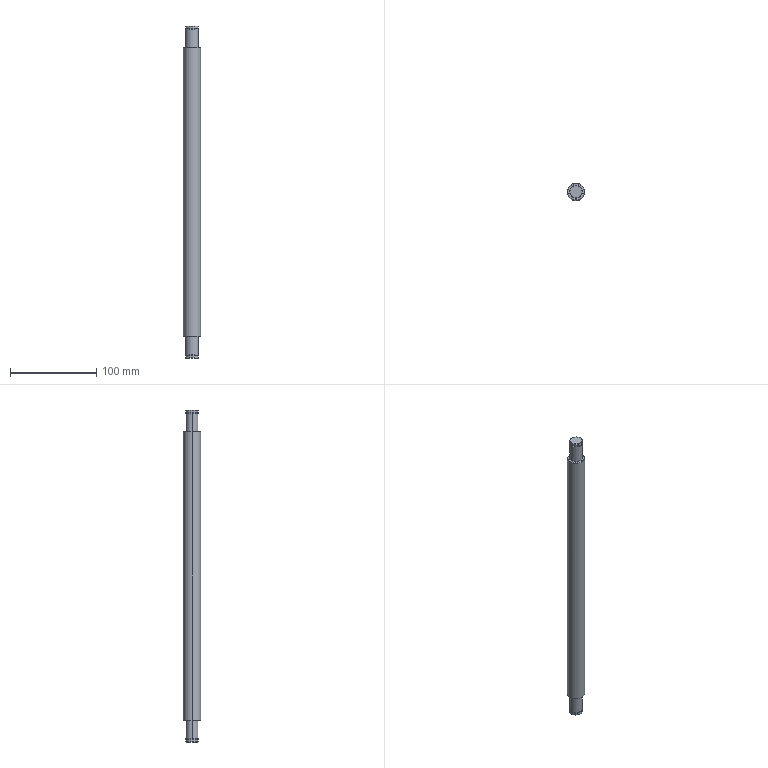Part | STEP file | 倍速链从动轴-0 | 1 solid | 30 faces | box 20 x 20 x 385.3 mm | volume 114081 mm3 | cylinder 14 | cone 8 | plane 8 | commonest cylinder face diameters 15 x8 13.8 x4 20 x2
STEP:
#1=CARTESIAN_POINT('',(-7.,0.,-192.65));
#2=VERTEX_POINT('',#1);
#3=CARTESIAN_POINT('',(7.,0.,-192.65));
#4=VERTEX_POINT('',#3);
#5=CARTESIAN_POINT('',(0.,0.,-192.65));
#6=DIRECTION('',(0.,0.,-1.));
#7=DIRECTION('',(-1.,0.,0.));
#8=AXIS2_PLACEMENT_3D('',#5,#6,#7);
#9=CIRCLE('',#8,7.);
#10=EDGE_CURVE('',#2,#4,#9,.T.);
#11=ORIENTED_EDGE('',*,*,#10,.F.);
#12=CARTESIAN_POINT('',(-7.5,0.,-192.15));
#13=VERTEX_POINT('',#12);
#14=CARTESIAN_POINT('',(-7.,0.,-192.65));
#15=DIRECTION('',(-0.7071,0.,0.7071));
#16=VECTOR('',#15,1000.);
#17=LINE('',#14,#16);
#18=EDGE_CURVE('',#2,#13,#17,.T.);
#19=ORIENTED_EDGE('',*,*,#18,.T.);
#20=CARTESIAN_POINT('',(7.5,0.,-192.15));
#21=VERTEX_POINT('',#20);
#22=CARTESIAN_POINT('',(0.,0.,-192.15));
#23=DIRECTION('',(0.,0.,1.));
#24=DIRECTION('',(-1.,0.,0.));
#25=AXIS2_PLACEMENT_3D('',#22,#23,#24);
#26=CIRCLE('',#25,7.5);
#27=EDGE_CURVE('',#21,#13,#26,.T.);
#28=ORIENTED_EDGE('',*,*,#27,.F.);
#29=CARTESIAN_POINT('',(7.,0.,-192.65));
#30=DIRECTION('',(0.7071,0.,0.7071));
#31=VECTOR('',#30,1000.);
#32=LINE('',#29,#31);
#33=EDGE_CURVE('',#4,#21,#32,.T.);
#34=ORIENTED_EDGE('',*,*,#33,.F.);
#35=EDGE_LOOP('',(#11,#19,#28,#34));
#36=FACE_OUTER_BOUND('',#35,.T.);
#37=CARTESIAN_POINT('',(0.,0.,-192.65));
#38=DIRECTION('',(0.,0.,1.));
#39=DIRECTION('',(1.,0.,0.));
#40=AXIS2_PLACEMENT_3D('',#37,#38,#39);
#41=CONICAL_SURFACE('',#40,7.,0.7854);
#42=ADVANCED_FACE('',(#36),#41,.T.);
#43=CARTESIAN_POINT('',(-9.5,0.,-167.65));
#44=VERTEX_POINT('',#43);
#45=CARTESIAN_POINT('',(9.5,0.,-167.65));
#46=VERTEX_POINT('',#45);
#47=CARTESIAN_POINT('',(0.,0.,-167.65));
#48=DIRECTION('',(0.,0.,-1.));
#49=DIRECTION('',(1.,0.,0.));
#50=AXIS2_PLACEMENT_3D('',#47,#48,#49);
#51=CIRCLE('',#50,9.5);
#52=EDGE_CURVE('',#44,#46,#51,.T.);
#53=ORIENTED_EDGE('',*,*,#52,.F.);
#54=CARTESIAN_POINT('',(-10.,0.,-167.15));
#55=VERTEX_POINT('',#54);
#56=CARTESIAN_POINT('',(-10.,0.,-167.15));
#57=DIRECTION('',(-0.7071,0.,0.7071));
#58=VECTOR('',#57,1000.);
#59=LINE('',#56,#58);
#60=EDGE_CURVE('',#44,#55,#59,.T.);
#61=ORIENTED_EDGE('',*,*,#60,.T.);
#62=CARTESIAN_POINT('',(10.,0.,-167.15));
#63=VERTEX_POINT('',#62);
#64=CARTESIAN_POINT('',(0.,0.,-167.15));
#65=DIRECTION('',(0.,0.,1.));
#66=DIRECTION('',(1.,0.,0.));
#67=AXIS2_PLACEMENT_3D('',#64,#65,#66);
#68=CIRCLE('',#67,10.);
#69=EDGE_CURVE('',#63,#55,#68,.T.);
#70=ORIENTED_EDGE('',*,*,#69,.F.);
#71=CARTESIAN_POINT('',(10.,0.,-167.15));
#72=DIRECTION('',(0.7071,0.,0.7071));
#73=VECTOR('',#72,1000.);
#74=LINE('',#71,#73);
#75=EDGE_CURVE('',#46,#63,#74,.T.);
#76=ORIENTED_EDGE('',*,*,#75,.F.);
#77=EDGE_LOOP('',(#53,#61,#70,#76));
#78=FACE_OUTER_BOUND('',#77,.T.);
#79=CARTESIAN_POINT('',(0.,0.,-167.15));
#80=DIRECTION('',(0.,0.,1.));
#81=DIRECTION('',(1.,0.,0.));
#82=AXIS2_PLACEMENT_3D('',#79,#80,#81);
#83=CONICAL_SURFACE('',#82,10.,0.7854);
#84=ADVANCED_FACE('',(#78),#83,.T.);
#85=CARTESIAN_POINT('',(9.5,0.,167.65));
#86=VERTEX_POINT('',#85);
#87=CARTESIAN_POINT('',(-9.5,0.,167.65));
#88=VERTEX_POINT('',#87);
#89=CARTESIAN_POINT('',(0.,0.,167.65));
#90=DIRECTION('',(0.,0.,1.));
#91=DIRECTION('',(1.,0.,0.));
#92=AXIS2_PLACEMENT_3D('',#89,#90,#91);
#93=CIRCLE('',#92,9.5);
#94=EDGE_CURVE('',#86,#88,#93,.T.);
#95=ORIENTED_EDGE('',*,*,#94,.F.);
#96=CARTESIAN_POINT('',(10.,0.,167.15));
#97=VERTEX_POINT('',#96);
#98=CARTESIAN_POINT('',(9.5,0.,167.65));
#99=DIRECTION('',(0.7071,0.,-0.7071));
#100=VECTOR('',#99,1000.);
#101=LINE('',#98,#100);
#102=EDGE_CURVE('',#86,#97,#101,.T.);
#103=ORIENTED_EDGE('',*,*,#102,.T.);
#104=CARTESIAN_POINT('',(-10.,0.,167.15));
#105=VERTEX_POINT('',#104);
#106=CARTESIAN_POINT('',(0.,0.,167.15));
#107=DIRECTION('',(0.,0.,-1.));
#108=DIRECTION('',(1.,0.,0.));
#109=AXIS2_PLACEMENT_3D('',#106,#107,#108);
#110=CIRCLE('',#109,10.);
#111=EDGE_CURVE('',#105,#97,#110,.T.);
#112=ORIENTED_EDGE('',*,*,#111,.F.);
#113=CARTESIAN_POINT('',(-9.5,0.,167.65));
#114=DIRECTION('',(-0.7071,0.,-0.7071));
#115=VECTOR('',#114,1000.);
#116=LINE('',#113,#115);
#117=EDGE_CURVE('',#88,#105,#116,.T.);
#118=ORIENTED_EDGE('',*,*,#117,.F.);
#119=EDGE_LOOP('',(#95,#103,#112,#118));
#120=FACE_OUTER_BOUND('',#119,.T.);
#121=CARTESIAN_POINT('',(0.,0.,167.65));
#122=DIRECTION('',(0.,0.,-1.));
#123=DIRECTION('',(-1.,0.,0.));
#124=AXIS2_PLACEMENT_3D('',#121,#122,#123);
#125=CONICAL_SURFACE('',#124,9.5,0.7854);
#126=ADVANCED_FACE('',(#120),#125,.T.);
#127=CARTESIAN_POINT('',(7.,0.,192.65));
#128=VERTEX_POINT('',#127);
#129=CARTESIAN_POINT('',(-7.,0.,192.65));
#130=VERTEX_POINT('',#129);
#131=CARTESIAN_POINT('',(0.,0.,192.65));
#132=DIRECTION('',(0.,0.,1.));
#133=DIRECTION('',(1.,0.,0.));
#134=AXIS2_PLACEMENT_3D('',#131,#132,#133);
#135=CIRCLE('',#134,7.);
#136=EDGE_CURVE('',#128,#130,#135,.T.);
#137=ORIENTED_EDGE('',*,*,#136,.F.);
#138=CARTESIAN_POINT('',(7.5,0.,192.15));
#139=VERTEX_POINT('',#138);
#140=CARTESIAN_POINT('',(7.5,0.,192.15));
#141=DIRECTION('',(0.7071,0.,-0.7071));
#142=VECTOR('',#141,1000.);
#143=LINE('',#140,#142);
#144=EDGE_CURVE('',#128,#139,#143,.T.);
#145=ORIENTED_EDGE('',*,*,#144,.T.);
#146=CARTESIAN_POINT('',(-7.5,0.,192.15));
#147=VERTEX_POINT('',#146);
#148=CARTESIAN_POINT('',(0.,0.,192.15));
#149=DIRECTION('',(0.,0.,-1.));
#150=DIRECTION('',(1.,0.,0.));
#151=AXIS2_PLACEMENT_3D('',#148,#149,#150);
#152=CIRCLE('',#151,7.5);
#153=EDGE_CURVE('',#147,#139,#152,.T.);
#154=ORIENTED_EDGE('',*,*,#153,.F.);
#155=CARTESIAN_POINT('',(-7.5,0.,192.15));
#156=DIRECTION('',(-0.7071,0.,-0.7071));
#157=VECTOR('',#156,1000.);
#158=LINE('',#155,#157);
#159=EDGE_CURVE('',#130,#147,#158,.T.);
#160=ORIENTED_EDGE('',*,*,#159,.F.);
#161=EDGE_LOOP('',(#137,#145,#154,#160));
#162=FACE_OUTER_BOUND('',#161,.T.);
#163=CARTESIAN_POINT('',(0.,0.,192.15));
#164=DIRECTION('',(0.,0.,-1.));
#165=DIRECTION('',(-1.,0.,0.));
#166=AXIS2_PLACEMENT_3D('',#163,#164,#165);
#167=CONICAL_SURFACE('',#166,7.5,0.7854);
#168=ADVANCED_FACE('',(#162),#167,.T.);
#169=ORIENTED_EDGE('',*,*,#27,.T.);
#170=CARTESIAN_POINT('',(-7.5,0.,-189.85));
#171=VERTEX_POINT('',#170);
#172=CARTESIAN_POINT('',(-7.5,0.,-192.65));
#173=DIRECTION('',(0.,0.,1.));
#174=VECTOR('',#173,1000.);
#175=LINE('',#172,#174);
#176=EDGE_CURVE('',#13,#171,#175,.T.);
#177=ORIENTED_EDGE('',*,*,#176,.T.);
#178=CARTESIAN_POINT('',(7.5,0.,-189.85));
#179=VERTEX_POINT('',#178);
#180=CARTESIAN_POINT('',(0.,0.,-189.85));
#181=DIRECTION('',(0.,0.,-1.));
#182=DIRECTION('',(-1.,0.,0.));
#183=AXIS2_PLACEMENT_3D('',#180,#181,#182);
#184=CIRCLE('',#183,7.5);
#185=EDGE_CURVE('',#171,#179,#184,.T.);
#186=ORIENTED_EDGE('',*,*,#185,.T.);
#187=CARTESIAN_POINT('',(7.5,0.,-192.65));
#188=DIRECTION('',(0.,0.,1.));
#189=VECTOR('',#188,1000.);
#190=LINE('',#187,#189);
#191=EDGE_CURVE('',#21,#179,#190,.T.);
#192=ORIENTED_EDGE('',*,*,#191,.F.);
#193=EDGE_LOOP('',(#169,#177,#186,#192));
#194=FACE_OUTER_BOUND('',#193,.T.);
#195=CARTESIAN_POINT('',(0.,0.,-192.65));
#196=DIRECTION('',(0.,0.,1.));
#197=DIRECTION('',(1.,0.,0.));
#198=AXIS2_PLACEMENT_3D('',#195,#196,#197);
#199=CYLINDRICAL_SURFACE('',#198,7.5);
#200=ADVANCED_FACE('',(#194),#199,.T.);
#201=CARTESIAN_POINT('',(6.9,0.,-189.85));
#202=VERTEX_POINT('',#201);
#203=CARTESIAN_POINT('',(-6.9,0.,-189.85));
#204=VERTEX_POINT('',#203);
#205=CARTESIAN_POINT('',(0.,0.,-189.85));
#206=DIRECTION('',(0.,0.,-1.));
#207=DIRECTION('',(-1.,0.,0.));
#208=AXIS2_PLACEMENT_3D('',#205,#206,#207);
#209=CIRCLE('',#208,6.9);
#210=EDGE_CURVE('',#202,#204,#209,.T.);
#211=ORIENTED_EDGE('',*,*,#210,.F.);
#212=CARTESIAN_POINT('',(6.9,0.,-188.65));
#213=VERTEX_POINT('',#212);
#214=CARTESIAN_POINT('',(6.9,0.,0.));
#215=DIRECTION('',(0.,0.,1.));
#216=VECTOR('',#215,1000.);
#217=LINE('',#214,#216);
#218=EDGE_CURVE('',#202,#213,#217,.T.);
#219=ORIENTED_EDGE('',*,*,#218,.T.);
#220=CARTESIAN_POINT('',(-6.9,0.,-188.65));
#221=VERTEX_POINT('',#220);
#222=CARTESIAN_POINT('',(0.,0.,-188.65));
#223=DIRECTION('',(0.,0.,-1.));
#224=DIRECTION('',(-1.,0.,0.));
#225=AXIS2_PLACEMENT_3D('',#222,#223,#224);
#226=CIRCLE('',#225,6.9);
#227=EDGE_CURVE('',#213,#221,#226,.T.);
#228=ORIENTED_EDGE('',*,*,#227,.T.);
#229=CARTESIAN_POINT('',(-6.9,0.,0.));
#230=DIRECTION('',(0.,0.,1.));
#231=VECTOR('',#230,1000.);
#232=LINE('',#229,#231);
#233=EDGE_CURVE('',#204,#221,#232,.T.);
#234=ORIENTED_EDGE('',*,*,#233,.F.);
#235=EDGE_LOOP('',(#211,#219,#228,#234));
#236=FACE_OUTER_BOUND('',#235,.T.);
#237=CARTESIAN_POINT('',(0.,0.,0.));
#238=DIRECTION('',(0.,0.,1.));
#239=DIRECTION('',(-1.,0.,0.));
#240=AXIS2_PLACEMENT_3D('',#237,#238,#239);
#241=CYLINDRICAL_SURFACE('',#240,6.9);
#242=ADVANCED_FACE('',(#236),#241,.T.);
#243=ORIENTED_EDGE('',*,*,#153,.T.);
#244=CARTESIAN_POINT('',(7.5,0.,189.85));
#245=VERTEX_POINT('',#244);
#246=CARTESIAN_POINT('',(7.5,0.,192.65));
#247=DIRECTION('',(0.,0.,-1.));
#248=VECTOR('',#247,1000.);
#249=LINE('',#246,#248);
#250=EDGE_CURVE('',#139,#245,#249,.T.);
#251=ORIENTED_EDGE('',*,*,#250,.T.);
#252=CARTESIAN_POINT('',(-7.5,0.,189.85));
#253=VERTEX_POINT('',#252);
#254=CARTESIAN_POINT('',(0.,0.,189.85));
#255=DIRECTION('',(0.,0.,-1.));
#256=DIRECTION('',(1.,0.,0.));
#257=AXIS2_PLACEMENT_3D('',#254,#255,#256);
#258=CIRCLE('',#257,7.5);
#259=EDGE_CURVE('',#253,#245,#258,.T.);
#260=ORIENTED_EDGE('',*,*,#259,.F.);
#261=CARTESIAN_POINT('',(-7.5,0.,192.65));
#262=DIRECTION('',(0.,0.,-1.));
#263=VECTOR('',#262,1000.);
#264=LINE('',#261,#263);
#265=EDGE_CURVE('',#147,#253,#264,.T.);
#266=ORIENTED_EDGE('',*,*,#265,.F.);
#267=EDGE_LOOP('',(#243,#251,#260,#266));
#268=FACE_OUTER_BOUND('',#267,.T.);
#269=CARTESIAN_POINT('',(0.,0.,192.65));
#270=DIRECTION('',(0.,0.,-1.));
#271=DIRECTION('',(-1.,0.,0.));
#272=AXIS2_PLACEMENT_3D('',#269,#270,#271);
#273=CYLINDRICAL_SURFACE('',#272,7.5);
#274=ADVANCED_FACE('',(#268),#273,.T.);
#275=CARTESIAN_POINT('',(-6.9,0.,189.85));
#276=VERTEX_POINT('',#275);
#277=CARTESIAN_POINT('',(6.9,0.,189.85));
#278=VERTEX_POINT('',#277);
#279=CARTESIAN_POINT('',(0.,0.,189.85));
#280=DIRECTION('',(0.,0.,-1.));
#281=DIRECTION('',(-1.,0.,0.));
#282=AXIS2_PLACEMENT_3D('',#279,#280,#281);
#283=CIRCLE('',#282,6.9);
#284=EDGE_CURVE('',#276,#278,#283,.T.);
#285=ORIENTED_EDGE('',*,*,#284,.T.);
#286=CARTESIAN_POINT('',(6.9,0.,188.65));
#287=VERTEX_POINT('',#286);
#288=CARTESIAN_POINT('',(6.9,0.,0.));
#289=DIRECTION('',(0.,0.,-1.));
#290=VECTOR('',#289,1000.);
#291=LINE('',#288,#290);
#292=EDGE_CURVE('',#278,#287,#291,.T.);
#293=ORIENTED_EDGE('',*,*,#292,.T.);
#294=CARTESIAN_POINT('',(-6.9,0.,188.65));
#295=VERTEX_POINT('',#294);
#296=CARTESIAN_POINT('',(0.,0.,188.65));
#297=DIRECTION('',(0.,0.,-1.));
#298=DIRECTION('',(-1.,0.,0.));
#299=AXIS2_PLACEMENT_3D('',#296,#297,#298);
#300=CIRCLE('',#299,6.9);
#301=EDGE_CURVE('',#295,#287,#300,.T.);
#302=ORIENTED_EDGE('',*,*,#301,.F.);
#303=CARTESIAN_POINT('',(-6.9,0.,0.));
#304=DIRECTION('',(0.,0.,-1.));
#305=VECTOR('',#304,1000.);
#306=LINE('',#303,#305);
#307=EDGE_CURVE('',#276,#295,#306,.T.);
#308=ORIENTED_EDGE('',*,*,#307,.F.);
#309=EDGE_LOOP('',(#285,#293,#302,#308));
#310=FACE_OUTER_BOUND('',#309,.T.);
#311=CARTESIAN_POINT('',(0.,0.,0.));
#312=DIRECTION('',(0.,0.,-1.));
#313=DIRECTION('',(-1.,0.,0.));
#314=AXIS2_PLACEMENT_3D('',#311,#312,#313);
#315=CYLINDRICAL_SURFACE('',#314,6.9);
#316=ADVANCED_FACE('',(#310),#315,.T.);
#317=CARTESIAN_POINT('',(7.5,0.,188.65));
#318=VERTEX_POINT('',#317);
#319=CARTESIAN_POINT('',(-7.5,0.,188.65));
#320=VERTEX_POINT('',#319);
#321=CARTESIAN_POINT('',(0.,0.,188.65));
#322=DIRECTION('',(0.,0.,1.));
#323=DIRECTION('',(-1.,0.,0.));
#324=AXIS2_PLACEMENT_3D('',#321,#322,#323);
#325=CIRCLE('',#324,7.5);
#326=EDGE_CURVE('',#318,#320,#325,.T.);
#327=ORIENTED_EDGE('',*,*,#326,.F.);
#328=CARTESIAN_POINT('',(7.5,0.,167.65));
#329=VERTEX_POINT('',#328);
#330=CARTESIAN_POINT('',(7.5,0.,192.65));
#331=DIRECTION('',(0.,0.,-1.));
#332=VECTOR('',#331,1000.);
#333=LINE('',#330,#332);
#334=EDGE_CURVE('',#318,#329,#333,.T.);
#335=ORIENTED_EDGE('',*,*,#334,.T.);
#336=CARTESIAN_POINT('',(-7.5,0.,167.65));
#337=VERTEX_POINT('',#336);
#338=CARTESIAN_POINT('',(0.,0.,167.65));
#339=DIRECTION('',(0.,0.,1.));
#340=DIRECTION('',(1.,0.,0.));
#341=AXIS2_PLACEMENT_3D('',#338,#339,#340);
#342=CIRCLE('',#341,7.5);
#343=EDGE_CURVE('',#329,#337,#342,.T.);
#344=ORIENTED_EDGE('',*,*,#343,.T.);
#345=CARTESIAN_POINT('',(-7.5,0.,192.65));
#346=DIRECTION('',(0.,0.,-1.));
#347=VECTOR('',#346,1000.);
#348=LINE('',#345,#347);
#349=EDGE_CURVE('',#320,#337,#348,.T.);
#350=ORIENTED_EDGE('',*,*,#349,.F.);
#351=EDGE_LOOP('',(#327,#335,#344,#350));
#352=FACE_OUTER_BOUND('',#351,.T.);
#353=CARTESIAN_POINT('',(0.,0.,192.65));
#354=DIRECTION('',(0.,0.,-1.));
#355=DIRECTION('',(-1.,0.,0.));
#356=AXIS2_PLACEMENT_3D('',#353,#354,#355);
#357=CYLINDRICAL_SURFACE('',#356,7.5);
#358=ADVANCED_FACE('',(#352),#357,.T.);
#359=CARTESIAN_POINT('',(7.5,0.,-188.65));
#360=VERTEX_POINT('',#359);
#361=CARTESIAN_POINT('',(-7.5,0.,-188.65));
#362=VERTEX_POINT('',#361);
#363=CARTESIAN_POINT('',(0.,0.,-188.65));
#364=DIRECTION('',(0.,0.,1.));
#365=DIRECTION('',(1.,0.,0.));
#366=AXIS2_PLACEMENT_3D('',#363,#364,#365);
#367=CIRCLE('',#366,7.5);
#368=EDGE_CURVE('',#360,#362,#367,.T.);
#369=ORIENTED_EDGE('',*,*,#368,.T.);
#370=CARTESIAN_POINT('',(-7.5,0.,-167.65));
#371=VERTEX_POINT('',#370);
#372=CARTESIAN_POINT('',(-7.5,0.,-192.65));
#373=DIRECTION('',(0.,0.,1.));
#374=VECTOR('',#373,1000.);
#375=LINE('',#372,#374);
#376=EDGE_CURVE('',#362,#371,#375,.T.);
#377=ORIENTED_EDGE('',*,*,#376,.T.);
#378=CARTESIAN_POINT('',(7.5,0.,-167.65));
#379=VERTEX_POINT('',#378);
#380=CARTESIAN_POINT('',(0.,0.,-167.65));
#381=DIRECTION('',(0.,0.,-1.));
#382=DIRECTION('',(1.,0.,0.));
#383=AXIS2_PLACEMENT_3D('',#380,#381,#382);
#384=CIRCLE('',#383,7.5);
#385=EDGE_CURVE('',#371,#379,#384,.T.);
#386=ORIENTED_EDGE('',*,*,#385,.T.);
#387=CARTESIAN_POINT('',(7.5,0.,-192.65));
#388=DIRECTION('',(0.,0.,1.));
#389=VECTOR('',#388,1000.);
#390=LINE('',#387,#389);
#391=EDGE_CURVE('',#360,#379,#390,.T.);
#392=ORIENTED_EDGE('',*,*,#391,.F.);
#393=EDGE_LOOP('',(#369,#377,#386,#392));
#394=FACE_OUTER_BOUND('',#393,.T.);
#395=CARTESIAN_POINT('',(0.,0.,-192.65));
#396=DIRECTION('',(0.,0.,1.));
#397=DIRECTION('',(1.,0.,0.));
#398=AXIS2_PLACEMENT_3D('',#395,#396,#397);
#399=CYLINDRICAL_SURFACE('',#398,7.5);
#400=ADVANCED_FACE('',(#394),#399,.T.);
#401=ORIENTED_EDGE('',*,*,#111,.T.);
#402=CARTESIAN_POINT('',(10.,0.,167.65));
#403=DIRECTION('',(0.,0.,-1.));
#404=VECTOR('',#403,1000.);
#405=LINE('',#402,#404);
#406=EDGE_CURVE('',#97,#63,#405,.T.);
#407=ORIENTED_EDGE('',*,*,#406,.T.);
#408=ORIENTED_EDGE('',*,*,#69,.T.);
#409=CARTESIAN_POINT('',(-10.,0.,167.65));
#410=DIRECTION('',(0.,0.,-1.));
#411=VECTOR('',#410,1000.);
#412=LINE('',#409,#411);
#413=EDGE_CURVE('',#105,#55,#412,.T.);
#414=ORIENTED_EDGE('',*,*,#413,.F.);
#415=EDGE_LOOP('',(#401,#407,#408,#414));
#416=FACE_OUTER_BOUND('',#415,.T.);
#417=CARTESIAN_POINT('',(0.,0.,167.65));
#418=DIRECTION('',(0.,0.,-1.));
#419=DIRECTION('',(-1.,0.,0.));
#420=AXIS2_PLACEMENT_3D('',#417,#418,#419);
#421=CYLINDRICAL_SURFACE('',#420,10.);
#422=ADVANCED_FACE('',(#416),#421,.T.);
#423=CARTESIAN_POINT('',(0.,0.,-167.65));
#424=DIRECTION('',(0.,0.,-1.));
#425=DIRECTION('',(1.,0.,0.));
#426=AXIS2_PLACEMENT_3D('',#423,#424,#425);
#427=CIRCLE('',#426,9.5);
#428=EDGE_CURVE('',#46,#44,#427,.T.);
#429=ORIENTED_EDGE('',*,*,#428,.T.);
#430=ORIENTED_EDGE('',*,*,#52,.T.);
#431=EDGE_LOOP('',(#429,#430));
#432=FACE_OUTER_BOUND('',#431,.T.);
#433=CARTESIAN_POINT('',(0.,0.,-167.65));
#434=DIRECTION('',(0.,0.,-1.));
#435=DIRECTION('',(1.,0.,0.));
#436=AXIS2_PLACEMENT_3D('',#433,#434,#435);
#437=CIRCLE('',#436,7.5);
#438=EDGE_CURVE('',#379,#371,#437,.T.);
#439=ORIENTED_EDGE('',*,*,#438,.F.);
#440=ORIENTED_EDGE('',*,*,#385,.F.);
#441=EDGE_LOOP('',(#439,#440));
#442=FACE_BOUND('',#441,.T.);
#443=CARTESIAN_POINT('',(0.,0.,-167.65));
#444=DIRECTION('',(0.,0.,1.));
#445=DIRECTION('',(1.,0.,0.));
#446=AXIS2_PLACEMENT_3D('',#443,#444,#445);
#447=PLANE('',#446);
#448=ADVANCED_FACE('',(#432,#442),#447,.F.);
#449=ORIENTED_EDGE('',*,*,#406,.F.);
#450=CARTESIAN_POINT('',(0.,0.,167.15));
#451=DIRECTION('',(0.,0.,-1.));
#452=DIRECTION('',(1.,0.,0.));
#453=AXIS2_PLACEMENT_3D('',#450,#451,#452);
#454=CIRCLE('',#453,10.);
#455=EDGE_CURVE('',#97,#105,#454,.T.);
#456=ORIENTED_EDGE('',*,*,#455,.T.);
#457=ORIENTED_EDGE('',*,*,#413,.T.);
#458=CARTESIAN_POINT('',(0.,0.,-167.15));
#459=DIRECTION('',(0.,0.,1.));
#460=DIRECTION('',(1.,0.,0.));
#461=AXIS2_PLACEMENT_3D('',#458,#459,#460);
#462=CIRCLE('',#461,10.);
#463=EDGE_CURVE('',#55,#63,#462,.T.);
#464=ORIENTED_EDGE('',*,*,#463,.T.);
#465=EDGE_LOOP('',(#449,#456,#457,#464));
#466=FACE_OUTER_BOUND('',#465,.T.);
#467=CARTESIAN_POINT('',(0.,0.,167.65));
#468=DIRECTION('',(0.,0.,-1.));
#469=DIRECTION('',(-1.,0.,0.));
#470=AXIS2_PLACEMENT_3D('',#467,#468,#469);
#471=CYLINDRICAL_SURFACE('',#470,10.);
#472=ADVANCED_FACE('',(#466),#471,.T.);
#473=CARTESIAN_POINT('',(0.,0.,167.65));
#474=DIRECTION('',(0.,0.,1.));
#475=DIRECTION('',(1.,0.,0.));
#476=AXIS2_PLACEMENT_3D('',#473,#474,#475);
#477=CIRCLE('',#476,9.5);
#478=EDGE_CURVE('',#88,#86,#477,.T.);
#479=ORIENTED_EDGE('',*,*,#478,.T.);
#480=ORIENTED_EDGE('',*,*,#94,.T.);
#481=EDGE_LOOP('',(#479,#480));
#482=FACE_OUTER_BOUND('',#481,.T.);
#483=CARTESIAN_POINT('',(0.,0.,167.65));
#484=DIRECTION('',(0.,0.,1.));
#485=DIRECTION('',(1.,0.,0.));
#486=AXIS2_PLACEMENT_3D('',#483,#484,#485);
#487=CIRCLE('',#486,7.5);
#488=EDGE_CURVE('',#337,#329,#487,.T.);
#489=ORIENTED_EDGE('',*,*,#488,.F.);
#490=ORIENTED_EDGE('',*,*,#343,.F.);
#491=EDGE_LOOP('',(#489,#490));
#492=FACE_BOUND('',#491,.T.);
#493=CARTESIAN_POINT('',(0.,0.,167.65));
#494=DIRECTION('',(0.,0.,1.));
#495=DIRECTION('',(1.,0.,0.));
#496=AXIS2_PLACEMENT_3D('',#493,#494,#495);
#497=PLANE('',#496);
#498=ADVANCED_FACE('',(#482,#492),#497,.T.);
#499=ORIENTED_EDGE('',*,*,#376,.F.);
#500=CARTESIAN_POINT('',(0.,0.,-188.65));
#501=DIRECTION('',(0.,0.,1.));
#502=DIRECTION('',(1.,0.,0.));
#503=AXIS2_PLACEMENT_3D('',#500,#501,#502);
#504=CIRCLE('',#503,7.5);
#505=EDGE_CURVE('',#362,#360,#504,.T.);
#506=ORIENTED_EDGE('',*,*,#505,.T.);
#507=ORIENTED_EDGE('',*,*,#391,.T.);
#508=ORIENTED_EDGE('',*,*,#438,.T.);
#509=EDGE_LOOP('',(#499,#506,#507,#508));
#510=FACE_OUTER_BOUND('',#509,.T.);
#511=CARTESIAN_POINT('',(0.,0.,-192.65));
#512=DIRECTION('',(0.,0.,1.));
#513=DIRECTION('',(1.,0.,0.));
#514=AXIS2_PLACEMENT_3D('',#511,#512,#513);
#515=CYLINDRICAL_SURFACE('',#514,7.5);
#516=ADVANCED_FACE('',(#510),#515,.T.);
#517=ORIENTED_EDGE('',*,*,#334,.F.);
#518=CARTESIAN_POINT('',(0.,0.,188.65));
#519=DIRECTION('',(0.,0.,1.));
#520=DIRECTION('',(-1.,0.,0.));
#521=AXIS2_PLACEMENT_3D('',#518,#519,#520);
#522=CIRCLE('',#521,7.5);
#523=EDGE_CURVE('',#320,#318,#522,.T.);
#524=ORIENTED_EDGE('',*,*,#523,.F.);
#525=ORIENTED_EDGE('',*,*,#349,.T.);
#526=ORIENTED_EDGE('',*,*,#488,.T.);
#527=EDGE_LOOP('',(#517,#524,#525,#526));
#528=FACE_OUTER_BOUND('',#527,.T.);
#529=CARTESIAN_POINT('',(0.,0.,192.65));
#530=DIRECTION('',(0.,0.,-1.));
#531=DIRECTION('',(-1.,0.,0.));
#532=AXIS2_PLACEMENT_3D('',#529,#530,#531);
#533=CYLINDRICAL_SURFACE('',#532,7.5);
#534=ADVANCED_FACE('',(#528),#533,.T.);
#535=ORIENTED_EDGE('',*,*,#259,.T.);
#536=CARTESIAN_POINT('',(0.,0.,189.85));
#537=DIRECTION('',(0.,0.,-1.));
#538=DIRECTION('',(1.,0.,0.));
#539=AXIS2_PLACEMENT_3D('',#536,#537,#538);
#540=CIRCLE('',#539,7.5);
#541=EDGE_CURVE('',#245,#253,#540,.T.);
#542=ORIENTED_EDGE('',*,*,#541,.T.);
#543=EDGE_LOOP('',(#535,#542));
#544=FACE_OUTER_BOUND('',#543,.T.);
#545=ORIENTED_EDGE('',*,*,#284,.F.);
#546=CARTESIAN_POINT('',(0.,0.,189.85));
#547=DIRECTION('',(0.,0.,-1.));
#548=DIRECTION('',(-1.,0.,0.));
#549=AXIS2_PLACEMENT_3D('',#546,#547,#548);
#550=CIRCLE('',#549,6.9);
#551=EDGE_CURVE('',#278,#276,#550,.T.);
#552=ORIENTED_EDGE('',*,*,#551,.F.);
#553=EDGE_LOOP('',(#545,#552));
#554=FACE_BOUND('',#553,.T.);
#555=CARTESIAN_POINT('',(-11.9,0.,189.85));
#556=DIRECTION('',(0.,0.,1.));
#557=DIRECTION('',(1.,0.,0.));
#558=AXIS2_PLACEMENT_3D('',#555,#556,#557);
#559=PLANE('',#558);
#560=ADVANCED_FACE('',(#544,#554),#559,.F.);
#561=ORIENTED_EDGE('',*,*,#292,.F.);
#562=ORIENTED_EDGE('',*,*,#551,.T.);
#563=ORIENTED_EDGE('',*,*,#307,.T.);
#564=CARTESIAN_POINT('',(0.,0.,188.65));
#565=DIRECTION('',(0.,0.,-1.));
#566=DIRECTION('',(-1.,0.,0.));
#567=AXIS2_PLACEMENT_3D('',#564,#565,#566);
#568=CIRCLE('',#567,6.9);
#569=EDGE_CURVE('',#287,#295,#568,.T.);
#570=ORIENTED_EDGE('',*,*,#569,.F.);
#571=EDGE_LOOP('',(#561,#562,#563,#570));
#572=FACE_OUTER_BOUND('',#571,.T.);
#573=CARTESIAN_POINT('',(0.,0.,0.));
#574=DIRECTION('',(0.,0.,-1.));
#575=DIRECTION('',(-1.,0.,0.));
#576=AXIS2_PLACEMENT_3D('',#573,#574,#575);
#577=CYLINDRICAL_SURFACE('',#576,6.9);
#578=ADVANCED_FACE('',(#572),#577,.T.);
#579=ORIENTED_EDGE('',*,*,#523,.T.);
#580=ORIENTED_EDGE('',*,*,#326,.T.);
#581=EDGE_LOOP('',(#579,#580));
#582=FACE_OUTER_BOUND('',#581,.T.);
#583=ORIENTED_EDGE('',*,*,#301,.T.);
#584=ORIENTED_EDGE('',*,*,#569,.T.);
#585=EDGE_LOOP('',(#583,#584));
#586=FACE_BOUND('',#585,.T.);
#587=CARTESIAN_POINT('',(-11.9,0.,188.65));
#588=DIRECTION('',(0.,0.,-1.));
#589=DIRECTION('',(-1.,0.,0.));
#590=AXIS2_PLACEMENT_3D('',#587,#588,#589);
#591=PLANE('',#590);
#592=ADVANCED_FACE('',(#582,#586),#591,.F.);
#593=CARTESIAN_POINT('',(0.,0.,192.65));
#594=DIRECTION('',(0.,0.,1.));
#595=DIRECTION('',(1.,0.,0.));
#596=AXIS2_PLACEMENT_3D('',#593,#594,#595);
#597=CIRCLE('',#596,7.);
#598=EDGE_CURVE('',#130,#128,#597,.T.);
#599=ORIENTED_EDGE('',*,*,#598,.T.);
#600=ORIENTED_EDGE('',*,*,#136,.T.);
#601=EDGE_LOOP('',(#599,#600));
#602=FACE_OUTER_BOUND('',#601,.T.);
#603=CARTESIAN_POINT('',(0.,0.,192.65));
#604=DIRECTION('',(0.,0.,1.));
#605=DIRECTION('',(-1.,0.,0.));
#606=AXIS2_PLACEMENT_3D('',#603,#604,#605);
#607=PLANE('',#606);
#608=ADVANCED_FACE('',(#602),#607,.T.);
#609=ORIENTED_EDGE('',*,*,#250,.F.);
#610=CARTESIAN_POINT('',(0.,0.,192.15));
#611=DIRECTION('',(0.,0.,-1.));
#612=DIRECTION('',(1.,0.,0.));
#613=AXIS2_PLACEMENT_3D('',#610,#611,#612);
#614=CIRCLE('',#613,7.5);
#615=EDGE_CURVE('',#139,#147,#614,.T.);
#616=ORIENTED_EDGE('',*,*,#615,.T.);
#617=ORIENTED_EDGE('',*,*,#265,.T.);
#618=ORIENTED_EDGE('',*,*,#541,.F.);
#619=EDGE_LOOP('',(#609,#616,#617,#618));
#620=FACE_OUTER_BOUND('',#619,.T.);
#621=CARTESIAN_POINT('',(0.,0.,192.65));
#622=DIRECTION('',(0.,0.,-1.));
#623=DIRECTION('',(-1.,0.,0.));
#624=AXIS2_PLACEMENT_3D('',#621,#622,#623);
#625=CYLINDRICAL_SURFACE('',#624,7.5);
#626=ADVANCED_FACE('',(#620),#625,.T.);
#627=CARTESIAN_POINT('',(0.,0.,-189.85));
#628=DIRECTION('',(0.,0.,-1.));
#629=DIRECTION('',(-1.,0.,0.));
#630=AXIS2_PLACEMENT_3D('',#627,#628,#629);
#631=CIRCLE('',#630,6.9);
#632=EDGE_CURVE('',#204,#202,#631,.T.);
#633=ORIENTED_EDGE('',*,*,#632,.T.);
#634=ORIENTED_EDGE('',*,*,#210,.T.);
#635=EDGE_LOOP('',(#633,#634));
#636=FACE_BOUND('',#635,.T.);
#637=CARTESIAN_POINT('',(0.,0.,-189.85));
#638=DIRECTION('',(0.,0.,-1.));
#639=DIRECTION('',(-1.,0.,0.));
#640=AXIS2_PLACEMENT_3D('',#637,#638,#639);
#641=CIRCLE('',#640,7.5);
#642=EDGE_CURVE('',#179,#171,#641,.T.);
#643=ORIENTED_EDGE('',*,*,#642,.F.);
#644=ORIENTED_EDGE('',*,*,#185,.F.);
#645=EDGE_LOOP('',(#643,#644));
#646=FACE_OUTER_BOUND('',#645,.T.);
#647=CARTESIAN_POINT('',(-11.9,0.,-189.85));
#648=DIRECTION('',(0.,0.,-1.));
#649=DIRECTION('',(1.,0.,0.));
#650=AXIS2_PLACEMENT_3D('',#647,#648,#649);
#651=PLANE('',#650);
#652=ADVANCED_FACE('',(#636,#646),#651,.F.);
#653=CARTESIAN_POINT('',(0.,0.,-188.65));
#654=DIRECTION('',(0.,0.,-1.));
#655=DIRECTION('',(-1.,0.,0.));
#656=AXIS2_PLACEMENT_3D('',#653,#654,#655);
#657=CIRCLE('',#656,6.9);
#658=EDGE_CURVE('',#221,#213,#657,.T.);
#659=ORIENTED_EDGE('',*,*,#658,.F.);
#660=ORIENTED_EDGE('',*,*,#227,.F.);
#661=EDGE_LOOP('',(#659,#660));
#662=FACE_BOUND('',#661,.T.);
#663=ORIENTED_EDGE('',*,*,#368,.F.);
#664=ORIENTED_EDGE('',*,*,#505,.F.);
#665=EDGE_LOOP('',(#663,#664));
#666=FACE_OUTER_BOUND('',#665,.T.);
#667=CARTESIAN_POINT('',(-11.9,0.,-188.65));
#668=DIRECTION('',(0.,0.,1.));
#669=DIRECTION('',(-1.,0.,0.));
#670=AXIS2_PLACEMENT_3D('',#667,#668,#669);
#671=PLANE('',#670);
#672=ADVANCED_FACE('',(#662,#666),#671,.F.);
#673=ORIENTED_EDGE('',*,*,#218,.F.);
#674=ORIENTED_EDGE('',*,*,#632,.F.);
#675=ORIENTED_EDGE('',*,*,#233,.T.);
#676=ORIENTED_EDGE('',*,*,#658,.T.);
#677=EDGE_LOOP('',(#673,#674,#675,#676));
#678=FACE_OUTER_BOUND('',#677,.T.);
#679=CARTESIAN_POINT('',(0.,0.,0.));
#680=DIRECTION('',(0.,0.,1.));
#681=DIRECTION('',(-1.,0.,0.));
#682=AXIS2_PLACEMENT_3D('',#679,#680,#681);
#683=CYLINDRICAL_SURFACE('',#682,6.9);
#684=ADVANCED_FACE('',(#678),#683,.T.);
#685=CARTESIAN_POINT('',(0.,0.,-192.65));
#686=DIRECTION('',(0.,0.,-1.));
#687=DIRECTION('',(-1.,0.,0.));
#688=AXIS2_PLACEMENT_3D('',#685,#686,#687);
#689=CIRCLE('',#688,7.);
#690=EDGE_CURVE('',#4,#2,#689,.T.);
#691=ORIENTED_EDGE('',*,*,#690,.T.);
#692=ORIENTED_EDGE('',*,*,#10,.T.);
#693=EDGE_LOOP('',(#691,#692));
#694=FACE_OUTER_BOUND('',#693,.T.);
#695=CARTESIAN_POINT('',(0.,0.,-192.65));
#696=DIRECTION('',(0.,0.,-1.));
#697=DIRECTION('',(-1.,0.,0.));
#698=AXIS2_PLACEMENT_3D('',#695,#696,#697);
#699=PLANE('',#698);
#700=ADVANCED_FACE('',(#694),#699,.T.);
#701=ORIENTED_EDGE('',*,*,#176,.F.);
#702=CARTESIAN_POINT('',(0.,0.,-192.15));
#703=DIRECTION('',(0.,0.,1.));
#704=DIRECTION('',(-1.,0.,0.));
#705=AXIS2_PLACEMENT_3D('',#702,#703,#704);
#706=CIRCLE('',#705,7.5);
#707=EDGE_CURVE('',#13,#21,#706,.T.);
#708=ORIENTED_EDGE('',*,*,#707,.T.);
#709=ORIENTED_EDGE('',*,*,#191,.T.);
#710=ORIENTED_EDGE('',*,*,#642,.T.);
#711=EDGE_LOOP('',(#701,#708,#709,#710));
#712=FACE_OUTER_BOUND('',#711,.T.);
#713=CARTESIAN_POINT('',(0.,0.,-192.65));
#714=DIRECTION('',(0.,0.,1.));
#715=DIRECTION('',(1.,0.,0.));
#716=AXIS2_PLACEMENT_3D('',#713,#714,#715);
#717=CYLINDRICAL_SURFACE('',#716,7.5);
#718=ADVANCED_FACE('',(#712),#717,.T.);
#719=ORIENTED_EDGE('',*,*,#144,.F.);
#720=ORIENTED_EDGE('',*,*,#598,.F.);
#721=ORIENTED_EDGE('',*,*,#159,.T.);
#722=ORIENTED_EDGE('',*,*,#615,.F.);
#723=EDGE_LOOP('',(#719,#720,#721,#722));
#724=FACE_OUTER_BOUND('',#723,.T.);
#725=CARTESIAN_POINT('',(0.,0.,192.15));
#726=DIRECTION('',(0.,0.,-1.));
#727=DIRECTION('',(-1.,0.,0.));
#728=AXIS2_PLACEMENT_3D('',#725,#726,#727);
#729=CONICAL_SURFACE('',#728,7.5,0.7854);
#730=ADVANCED_FACE('',(#724),#729,.T.);
#731=ORIENTED_EDGE('',*,*,#102,.F.);
#732=ORIENTED_EDGE('',*,*,#478,.F.);
#733=ORIENTED_EDGE('',*,*,#117,.T.);
#734=ORIENTED_EDGE('',*,*,#455,.F.);
#735=EDGE_LOOP('',(#731,#732,#733,#734));
#736=FACE_OUTER_BOUND('',#735,.T.);
#737=CARTESIAN_POINT('',(0.,0.,167.65));
#738=DIRECTION('',(0.,0.,-1.));
#739=DIRECTION('',(-1.,0.,0.));
#740=AXIS2_PLACEMENT_3D('',#737,#738,#739);
#741=CONICAL_SURFACE('',#740,9.5,0.7854);
#742=ADVANCED_FACE('',(#736),#741,.T.);
#743=ORIENTED_EDGE('',*,*,#60,.F.);
#744=ORIENTED_EDGE('',*,*,#428,.F.);
#745=ORIENTED_EDGE('',*,*,#75,.T.);
#746=ORIENTED_EDGE('',*,*,#463,.F.);
#747=EDGE_LOOP('',(#743,#744,#745,#746));
#748=FACE_OUTER_BOUND('',#747,.T.);
#749=CARTESIAN_POINT('',(0.,0.,-167.15));
#750=DIRECTION('',(0.,0.,1.));
#751=DIRECTION('',(1.,0.,0.));
#752=AXIS2_PLACEMENT_3D('',#749,#750,#751);
#753=CONICAL_SURFACE('',#752,10.,0.7854);
#754=ADVANCED_FACE('',(#748),#753,.T.);
#755=ORIENTED_EDGE('',*,*,#18,.F.);
#756=ORIENTED_EDGE('',*,*,#690,.F.);
#757=ORIENTED_EDGE('',*,*,#33,.T.);
#758=ORIENTED_EDGE('',*,*,#707,.F.);
#759=EDGE_LOOP('',(#755,#756,#757,#758));
#760=FACE_OUTER_BOUND('',#759,.T.);
#761=CARTESIAN_POINT('',(0.,0.,-192.65));
#762=DIRECTION('',(0.,0.,1.));
#763=DIRECTION('',(1.,0.,0.));
#764=AXIS2_PLACEMENT_3D('',#761,#762,#763);
#765=CONICAL_SURFACE('',#764,7.,0.7854);
#766=ADVANCED_FACE('',(#760),#765,.T.);
#767=CLOSED_SHELL('',(#42,#84,#126,#168,#200,#242,#274,#316,#358,#400,#422,#448,#472,#498,#516,#534,#560,#578,#592,#608,#626,#652,#672,#684,#700,#718,#730,#742,#754,#766));
#768=MANIFOLD_SOLID_BREP('',#767);
#769=CARTESIAN_POINT('',(0.,0.,0.));
#770=DIRECTION('',(0.,0.,1.));
#771=DIRECTION('',(1.,0.,0.));
#772=AXIS2_PLACEMENT_3D('',#769,#770,#771);
#773=(LENGTH_UNIT()NAMED_UNIT(*)SI_UNIT(.MILLI.,.METRE.));
#774=UNCERTAINTY_MEASURE_WITH_UNIT(LENGTH_MEASURE(0.00001),#773,'','');
#775=(NAMED_UNIT(*)PLANE_ANGLE_UNIT()SI_UNIT($,.RADIAN.));
#776=(NAMED_UNIT(*)SI_UNIT($,.STERADIAN.)SOLID_ANGLE_UNIT());
#777=(GEOMETRIC_REPRESENTATION_CONTEXT(3)GLOBAL_UNCERTAINTY_ASSIGNED_CONTEXT((#774))GLOBAL_UNIT_ASSIGNED_CONTEXT((#773,#775,#776))REPRESENTATION_CONTEXT('',''));
#778=ADVANCED_BREP_SHAPE_REPRESENTATION('',(#768,#772),#777);